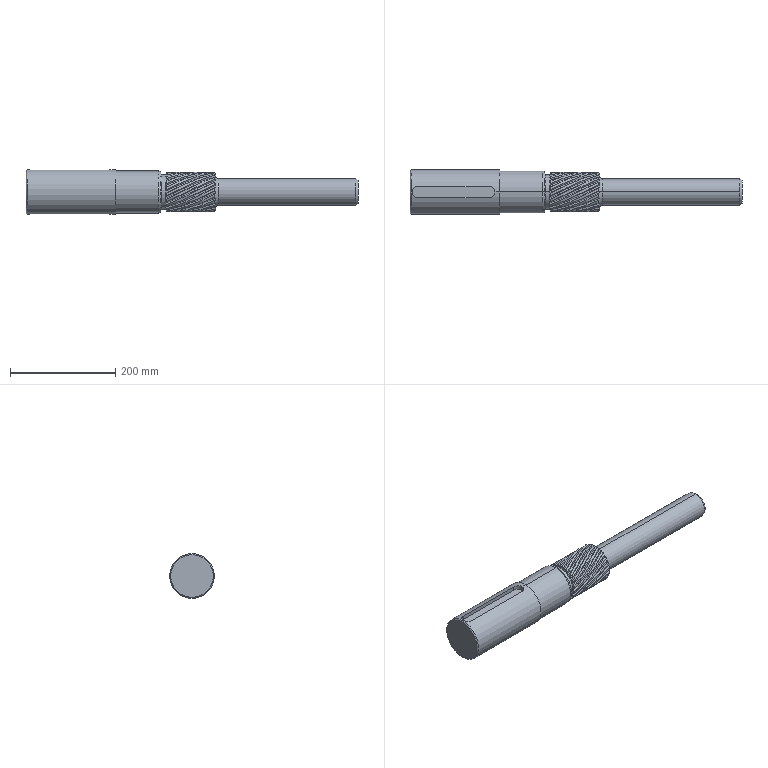Part | SolidWorks | features ICE 6, Chamfer 4, Fillet 2, CirPattern 1, Extrusion 1, Helix 1, HoleWzd 1, MirrorPattern 1, SweepCut 1 | 1 solid | 146 faces | box 630 x 85 x 85 mm | volume 2283899 mm3 | spline 60 | cylinder 40 | cone 28 | plane 12 | torus 6 | commonest cylinder face diameters 75 x24 22 x6 6.8 x2 50 x2 65 x2 80 x2